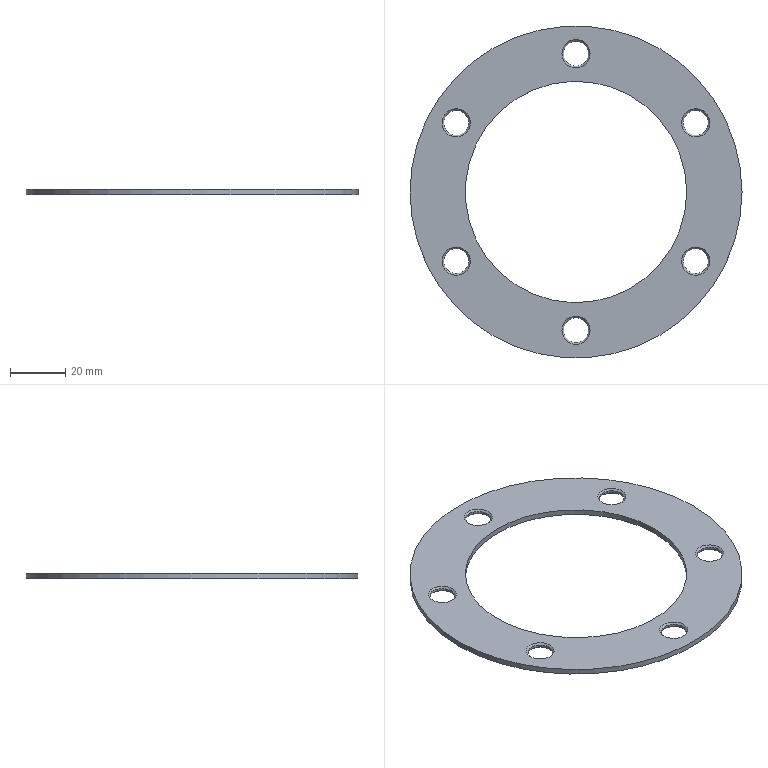Part | NX | 1 solid | 22 faces | box 120 x 120 x 2 mm | volume 11739 mm3 | cone 12 | cylinder 8 | plane 2 | commonest cylinder face diameters 9 x6 80 x1 120 x1
STEP:
#1=CARTESIAN_POINT('',(-41.051,28.897,1.4));
#2=VERTEX_POINT('',#1);
#3=CARTESIAN_POINT('',(-43.301,25.,1.4));
#4=DIRECTION('',(0.,0.,1.));
#5=DIRECTION('',(0.5,0.866,0.));
#6=AXIS2_PLACEMENT_3D('',#3,#4,#5);
#7=CIRCLE('',#6,4.5);
#8=EDGE_CURVE('',#2,#2,#7,.T.);
#9=ORIENTED_EDGE('',*,*,#8,.T.);
#10=EDGE_LOOP('',(#9));
#11=FACE_BOUND('',#10,.T.);
#12=CARTESIAN_POINT('',(-41.051,28.897,0.6));
#13=VERTEX_POINT('',#12);
#14=CARTESIAN_POINT('',(-43.301,25.,0.6));
#15=DIRECTION('',(0.,0.,-1.));
#16=DIRECTION('',(0.5,0.866,0.));
#17=AXIS2_PLACEMENT_3D('',#14,#15,#16);
#18=CIRCLE('',#17,4.5);
#19=EDGE_CURVE('',#13,#13,#18,.T.);
#20=ORIENTED_EDGE('',*,*,#19,.T.);
#21=EDGE_LOOP('',(#20));
#22=FACE_BOUND('',#21,.T.);
#23=CARTESIAN_POINT('',(-43.301,25.,0.));
#24=DIRECTION('',(0.,0.,1.));
#25=DIRECTION('',(-0.5,-0.866,0.));
#26=AXIS2_PLACEMENT_3D('',#23,#24,#25);
#27=CYLINDRICAL_SURFACE('',#26,4.5);
#28=ADVANCED_FACE('',(#11,#22),#27,.F.);
#29=CARTESIAN_POINT('',(-40.751,29.417,2.));
#30=VERTEX_POINT('',#29);
#31=CARTESIAN_POINT('',(-43.301,25.,2.));
#32=DIRECTION('',(0.,0.,-1.));
#33=DIRECTION('',(0.5,0.866,0.));
#34=AXIS2_PLACEMENT_3D('',#31,#32,#33);
#35=CIRCLE('',#34,5.1);
#36=EDGE_CURVE('',#30,#30,#35,.T.);
#37=ORIENTED_EDGE('',*,*,#36,.F.);
#38=EDGE_LOOP('',(#37));
#39=FACE_BOUND('',#38,.T.);
#40=ORIENTED_EDGE('',*,*,#8,.F.);
#41=EDGE_LOOP('',(#40));
#42=FACE_BOUND('',#41,.T.);
#43=CARTESIAN_POINT('',(-43.301,25.,1.4));
#44=DIRECTION('',(0.,0.,1.));
#45=DIRECTION('',(-0.5,-0.866,0.));
#46=AXIS2_PLACEMENT_3D('',#43,#44,#45);
#47=CONICAL_SURFACE('',#46,4.5,45.);
#48=ADVANCED_FACE('',(#39,#42),#47,.F.);
#49=ORIENTED_EDGE('',*,*,#19,.F.);
#50=EDGE_LOOP('',(#49));
#51=FACE_BOUND('',#50,.T.);
#52=CARTESIAN_POINT('',(-40.751,29.417,0.));
#53=VERTEX_POINT('',#52);
#54=CARTESIAN_POINT('',(-43.301,25.,0.));
#55=DIRECTION('',(0.,0.,1.));
#56=DIRECTION('',(0.5,0.866,0.));
#57=AXIS2_PLACEMENT_3D('',#54,#55,#56);
#58=CIRCLE('',#57,5.1);
#59=EDGE_CURVE('',#53,#53,#58,.T.);
#60=ORIENTED_EDGE('',*,*,#59,.F.);
#61=EDGE_LOOP('',(#60));
#62=FACE_BOUND('',#61,.T.);
#63=CARTESIAN_POINT('',(-43.301,25.,0.));
#64=DIRECTION('',(0.,0.,-1.));
#65=DIRECTION('',(0.5,0.866,0.));
#66=AXIS2_PLACEMENT_3D('',#63,#64,#65);
#67=CONICAL_SURFACE('',#66,5.1,45.);
#68=ADVANCED_FACE('',(#51,#62),#67,.F.);
#69=CARTESIAN_POINT('',(-45.551,-21.103,1.4));
#70=VERTEX_POINT('',#69);
#71=CARTESIAN_POINT('',(-43.301,-25.,1.4));
#72=DIRECTION('',(0.,0.,1.));
#73=DIRECTION('',(-0.5,0.866,0.));
#74=AXIS2_PLACEMENT_3D('',#71,#72,#73);
#75=CIRCLE('',#74,4.5);
#76=EDGE_CURVE('',#70,#70,#75,.T.);
#77=ORIENTED_EDGE('',*,*,#76,.T.);
#78=EDGE_LOOP('',(#77));
#79=FACE_BOUND('',#78,.T.);
#80=CARTESIAN_POINT('',(-45.551,-21.103,0.6));
#81=VERTEX_POINT('',#80);
#82=CARTESIAN_POINT('',(-43.301,-25.,0.6));
#83=DIRECTION('',(0.,0.,-1.));
#84=DIRECTION('',(-0.5,0.866,0.));
#85=AXIS2_PLACEMENT_3D('',#82,#83,#84);
#86=CIRCLE('',#85,4.5);
#87=EDGE_CURVE('',#81,#81,#86,.T.);
#88=ORIENTED_EDGE('',*,*,#87,.T.);
#89=EDGE_LOOP('',(#88));
#90=FACE_BOUND('',#89,.T.);
#91=CARTESIAN_POINT('',(-43.301,-25.,0.));
#92=DIRECTION('',(0.,0.,1.));
#93=DIRECTION('',(0.5,-0.866,0.));
#94=AXIS2_PLACEMENT_3D('',#91,#92,#93);
#95=CYLINDRICAL_SURFACE('',#94,4.5);
#96=ADVANCED_FACE('',(#79,#90),#95,.F.);
#97=CARTESIAN_POINT('',(-45.851,-20.583,2.));
#98=VERTEX_POINT('',#97);
#99=CARTESIAN_POINT('',(-43.301,-25.,2.));
#100=DIRECTION('',(0.,0.,-1.));
#101=DIRECTION('',(-0.5,0.866,0.));
#102=AXIS2_PLACEMENT_3D('',#99,#100,#101);
#103=CIRCLE('',#102,5.1);
#104=EDGE_CURVE('',#98,#98,#103,.T.);
#105=ORIENTED_EDGE('',*,*,#104,.F.);
#106=EDGE_LOOP('',(#105));
#107=FACE_BOUND('',#106,.T.);
#108=ORIENTED_EDGE('',*,*,#76,.F.);
#109=EDGE_LOOP('',(#108));
#110=FACE_BOUND('',#109,.T.);
#111=CARTESIAN_POINT('',(-43.301,-25.,1.4));
#112=DIRECTION('',(0.,0.,1.));
#113=DIRECTION('',(0.5,-0.866,0.));
#114=AXIS2_PLACEMENT_3D('',#111,#112,#113);
#115=CONICAL_SURFACE('',#114,4.5,45.);
#116=ADVANCED_FACE('',(#107,#110),#115,.F.);
#117=ORIENTED_EDGE('',*,*,#87,.F.);
#118=EDGE_LOOP('',(#117));
#119=FACE_BOUND('',#118,.T.);
#120=CARTESIAN_POINT('',(-45.851,-20.583,0.));
#121=VERTEX_POINT('',#120);
#122=CARTESIAN_POINT('',(-43.301,-25.,0.));
#123=DIRECTION('',(0.,0.,1.));
#124=DIRECTION('',(-0.5,0.866,0.));
#125=AXIS2_PLACEMENT_3D('',#122,#123,#124);
#126=CIRCLE('',#125,5.1);
#127=EDGE_CURVE('',#121,#121,#126,.T.);
#128=ORIENTED_EDGE('',*,*,#127,.F.);
#129=EDGE_LOOP('',(#128));
#130=FACE_BOUND('',#129,.T.);
#131=CARTESIAN_POINT('',(-43.301,-25.,0.));
#132=DIRECTION('',(0.,0.,-1.));
#133=DIRECTION('',(-0.5,0.866,0.));
#134=AXIS2_PLACEMENT_3D('',#131,#132,#133);
#135=CONICAL_SURFACE('',#134,5.1,45.);
#136=ADVANCED_FACE('',(#119,#130),#135,.F.);
#137=CARTESIAN_POINT('',(-4.5,-50.,1.4));
#138=VERTEX_POINT('',#137);
#139=CARTESIAN_POINT('',(0.,-50.,1.4));
#140=DIRECTION('',(0.,0.,1.));
#141=DIRECTION('',(-1.,0.,0.));
#142=AXIS2_PLACEMENT_3D('',#139,#140,#141);
#143=CIRCLE('',#142,4.5);
#144=EDGE_CURVE('',#138,#138,#143,.T.);
#145=ORIENTED_EDGE('',*,*,#144,.T.);
#146=EDGE_LOOP('',(#145));
#147=FACE_BOUND('',#146,.T.);
#148=CARTESIAN_POINT('',(-4.5,-50.,0.6));
#149=VERTEX_POINT('',#148);
#150=CARTESIAN_POINT('',(0.,-50.,0.6));
#151=DIRECTION('',(0.,0.,-1.));
#152=DIRECTION('',(-1.,0.,0.));
#153=AXIS2_PLACEMENT_3D('',#150,#151,#152);
#154=CIRCLE('',#153,4.5);
#155=EDGE_CURVE('',#149,#149,#154,.T.);
#156=ORIENTED_EDGE('',*,*,#155,.T.);
#157=EDGE_LOOP('',(#156));
#158=FACE_BOUND('',#157,.T.);
#159=CARTESIAN_POINT('',(0.,-50.,0.));
#160=DIRECTION('',(0.,0.,1.));
#161=DIRECTION('',(1.,0.,0.));
#162=AXIS2_PLACEMENT_3D('',#159,#160,#161);
#163=CYLINDRICAL_SURFACE('',#162,4.5);
#164=ADVANCED_FACE('',(#147,#158),#163,.F.);
#165=CARTESIAN_POINT('',(-5.1,-50.,2.));
#166=VERTEX_POINT('',#165);
#167=CARTESIAN_POINT('',(0.,-50.,2.));
#168=DIRECTION('',(0.,0.,-1.));
#169=DIRECTION('',(-1.,0.,0.));
#170=AXIS2_PLACEMENT_3D('',#167,#168,#169);
#171=CIRCLE('',#170,5.1);
#172=EDGE_CURVE('',#166,#166,#171,.T.);
#173=ORIENTED_EDGE('',*,*,#172,.F.);
#174=EDGE_LOOP('',(#173));
#175=FACE_BOUND('',#174,.T.);
#176=ORIENTED_EDGE('',*,*,#144,.F.);
#177=EDGE_LOOP('',(#176));
#178=FACE_BOUND('',#177,.T.);
#179=CARTESIAN_POINT('',(0.,-50.,1.4));
#180=DIRECTION('',(0.,0.,1.));
#181=DIRECTION('',(1.,0.,0.));
#182=AXIS2_PLACEMENT_3D('',#179,#180,#181);
#183=CONICAL_SURFACE('',#182,4.5,45.);
#184=ADVANCED_FACE('',(#175,#178),#183,.F.);
#185=ORIENTED_EDGE('',*,*,#155,.F.);
#186=EDGE_LOOP('',(#185));
#187=FACE_BOUND('',#186,.T.);
#188=CARTESIAN_POINT('',(-5.1,-50.,0.));
#189=VERTEX_POINT('',#188);
#190=CARTESIAN_POINT('',(0.,-50.,0.));
#191=DIRECTION('',(0.,0.,1.));
#192=DIRECTION('',(-1.,0.,0.));
#193=AXIS2_PLACEMENT_3D('',#190,#191,#192);
#194=CIRCLE('',#193,5.1);
#195=EDGE_CURVE('',#189,#189,#194,.T.);
#196=ORIENTED_EDGE('',*,*,#195,.F.);
#197=EDGE_LOOP('',(#196));
#198=FACE_BOUND('',#197,.T.);
#199=CARTESIAN_POINT('',(0.,-50.,0.));
#200=DIRECTION('',(0.,0.,-1.));
#201=DIRECTION('',(-1.,0.,0.));
#202=AXIS2_PLACEMENT_3D('',#199,#200,#201);
#203=CONICAL_SURFACE('',#202,5.1,45.);
#204=ADVANCED_FACE('',(#187,#198),#203,.F.);
#205=CARTESIAN_POINT('',(41.051,-28.897,1.4));
#206=VERTEX_POINT('',#205);
#207=CARTESIAN_POINT('',(43.301,-25.,1.4));
#208=DIRECTION('',(0.,0.,1.));
#209=DIRECTION('',(-0.5,-0.866,0.));
#210=AXIS2_PLACEMENT_3D('',#207,#208,#209);
#211=CIRCLE('',#210,4.5);
#212=EDGE_CURVE('',#206,#206,#211,.T.);
#213=ORIENTED_EDGE('',*,*,#212,.T.);
#214=EDGE_LOOP('',(#213));
#215=FACE_BOUND('',#214,.T.);
#216=CARTESIAN_POINT('',(41.051,-28.897,0.6));
#217=VERTEX_POINT('',#216);
#218=CARTESIAN_POINT('',(43.301,-25.,0.6));
#219=DIRECTION('',(0.,0.,-1.));
#220=DIRECTION('',(-0.5,-0.866,0.));
#221=AXIS2_PLACEMENT_3D('',#218,#219,#220);
#222=CIRCLE('',#221,4.5);
#223=EDGE_CURVE('',#217,#217,#222,.T.);
#224=ORIENTED_EDGE('',*,*,#223,.T.);
#225=EDGE_LOOP('',(#224));
#226=FACE_BOUND('',#225,.T.);
#227=CARTESIAN_POINT('',(43.301,-25.,0.));
#228=DIRECTION('',(0.,0.,1.));
#229=DIRECTION('',(0.5,0.866,0.));
#230=AXIS2_PLACEMENT_3D('',#227,#228,#229);
#231=CYLINDRICAL_SURFACE('',#230,4.5);
#232=ADVANCED_FACE('',(#215,#226),#231,.F.);
#233=CARTESIAN_POINT('',(40.751,-29.417,2.));
#234=VERTEX_POINT('',#233);
#235=CARTESIAN_POINT('',(43.301,-25.,2.));
#236=DIRECTION('',(0.,0.,-1.));
#237=DIRECTION('',(-0.5,-0.866,0.));
#238=AXIS2_PLACEMENT_3D('',#235,#236,#237);
#239=CIRCLE('',#238,5.1);
#240=EDGE_CURVE('',#234,#234,#239,.T.);
#241=ORIENTED_EDGE('',*,*,#240,.F.);
#242=EDGE_LOOP('',(#241));
#243=FACE_BOUND('',#242,.T.);
#244=ORIENTED_EDGE('',*,*,#212,.F.);
#245=EDGE_LOOP('',(#244));
#246=FACE_BOUND('',#245,.T.);
#247=CARTESIAN_POINT('',(43.301,-25.,1.4));
#248=DIRECTION('',(0.,0.,1.));
#249=DIRECTION('',(0.5,0.866,0.));
#250=AXIS2_PLACEMENT_3D('',#247,#248,#249);
#251=CONICAL_SURFACE('',#250,4.5,45.);
#252=ADVANCED_FACE('',(#243,#246),#251,.F.);
#253=ORIENTED_EDGE('',*,*,#223,.F.);
#254=EDGE_LOOP('',(#253));
#255=FACE_BOUND('',#254,.T.);
#256=CARTESIAN_POINT('',(40.751,-29.417,0.));
#257=VERTEX_POINT('',#256);
#258=CARTESIAN_POINT('',(43.301,-25.,0.));
#259=DIRECTION('',(0.,0.,1.));
#260=DIRECTION('',(-0.5,-0.866,0.));
#261=AXIS2_PLACEMENT_3D('',#258,#259,#260);
#262=CIRCLE('',#261,5.1);
#263=EDGE_CURVE('',#257,#257,#262,.T.);
#264=ORIENTED_EDGE('',*,*,#263,.F.);
#265=EDGE_LOOP('',(#264));
#266=FACE_BOUND('',#265,.T.);
#267=CARTESIAN_POINT('',(43.301,-25.,0.));
#268=DIRECTION('',(0.,0.,-1.));
#269=DIRECTION('',(-0.5,-0.866,0.));
#270=AXIS2_PLACEMENT_3D('',#267,#268,#269);
#271=CONICAL_SURFACE('',#270,5.1,45.);
#272=ADVANCED_FACE('',(#255,#266),#271,.F.);
#273=CARTESIAN_POINT('',(45.551,21.103,1.4));
#274=VERTEX_POINT('',#273);
#275=CARTESIAN_POINT('',(43.301,25.,1.4));
#276=DIRECTION('',(0.,0.,1.));
#277=DIRECTION('',(0.5,-0.866,0.));
#278=AXIS2_PLACEMENT_3D('',#275,#276,#277);
#279=CIRCLE('',#278,4.5);
#280=EDGE_CURVE('',#274,#274,#279,.T.);
#281=ORIENTED_EDGE('',*,*,#280,.T.);
#282=EDGE_LOOP('',(#281));
#283=FACE_BOUND('',#282,.T.);
#284=CARTESIAN_POINT('',(45.551,21.103,0.6));
#285=VERTEX_POINT('',#284);
#286=CARTESIAN_POINT('',(43.301,25.,0.6));
#287=DIRECTION('',(0.,0.,-1.));
#288=DIRECTION('',(0.5,-0.866,0.));
#289=AXIS2_PLACEMENT_3D('',#286,#287,#288);
#290=CIRCLE('',#289,4.5);
#291=EDGE_CURVE('',#285,#285,#290,.T.);
#292=ORIENTED_EDGE('',*,*,#291,.T.);
#293=EDGE_LOOP('',(#292));
#294=FACE_BOUND('',#293,.T.);
#295=CARTESIAN_POINT('',(43.301,25.,0.));
#296=DIRECTION('',(0.,0.,1.));
#297=DIRECTION('',(-0.5,0.866,0.));
#298=AXIS2_PLACEMENT_3D('',#295,#296,#297);
#299=CYLINDRICAL_SURFACE('',#298,4.5);
#300=ADVANCED_FACE('',(#283,#294),#299,.F.);
#301=CARTESIAN_POINT('',(45.851,20.583,2.));
#302=VERTEX_POINT('',#301);
#303=CARTESIAN_POINT('',(43.301,25.,2.));
#304=DIRECTION('',(0.,0.,-1.));
#305=DIRECTION('',(0.5,-0.866,0.));
#306=AXIS2_PLACEMENT_3D('',#303,#304,#305);
#307=CIRCLE('',#306,5.1);
#308=EDGE_CURVE('',#302,#302,#307,.T.);
#309=ORIENTED_EDGE('',*,*,#308,.F.);
#310=EDGE_LOOP('',(#309));
#311=FACE_BOUND('',#310,.T.);
#312=ORIENTED_EDGE('',*,*,#280,.F.);
#313=EDGE_LOOP('',(#312));
#314=FACE_BOUND('',#313,.T.);
#315=CARTESIAN_POINT('',(43.301,25.,1.4));
#316=DIRECTION('',(0.,0.,1.));
#317=DIRECTION('',(-0.5,0.866,0.));
#318=AXIS2_PLACEMENT_3D('',#315,#316,#317);
#319=CONICAL_SURFACE('',#318,4.5,45.);
#320=ADVANCED_FACE('',(#311,#314),#319,.F.);
#321=ORIENTED_EDGE('',*,*,#291,.F.);
#322=EDGE_LOOP('',(#321));
#323=FACE_BOUND('',#322,.T.);
#324=CARTESIAN_POINT('',(45.851,20.583,0.));
#325=VERTEX_POINT('',#324);
#326=CARTESIAN_POINT('',(43.301,25.,0.));
#327=DIRECTION('',(0.,0.,1.));
#328=DIRECTION('',(0.5,-0.866,0.));
#329=AXIS2_PLACEMENT_3D('',#326,#327,#328);
#330=CIRCLE('',#329,5.1);
#331=EDGE_CURVE('',#325,#325,#330,.T.);
#332=ORIENTED_EDGE('',*,*,#331,.F.);
#333=EDGE_LOOP('',(#332));
#334=FACE_BOUND('',#333,.T.);
#335=CARTESIAN_POINT('',(43.301,25.,0.));
#336=DIRECTION('',(0.,0.,-1.));
#337=DIRECTION('',(0.5,-0.866,0.));
#338=AXIS2_PLACEMENT_3D('',#335,#336,#337);
#339=CONICAL_SURFACE('',#338,5.1,45.);
#340=ADVANCED_FACE('',(#323,#334),#339,.F.);
#341=CARTESIAN_POINT('',(60.,0.,2.));
#342=VERTEX_POINT('',#341);
#343=CARTESIAN_POINT('',(0.,0.,2.));
#344=DIRECTION('',(0.,0.,1.));
#345=DIRECTION('',(1.,0.,0.));
#346=AXIS2_PLACEMENT_3D('',#343,#344,#345);
#347=CIRCLE('',#346,60.);
#348=EDGE_CURVE('',#342,#342,#347,.T.);
#349=ORIENTED_EDGE('',*,*,#348,.F.);
#350=EDGE_LOOP('',(#349));
#351=FACE_BOUND('',#350,.T.);
#352=CARTESIAN_POINT('',(60.,0.,0.));
#353=VERTEX_POINT('',#352);
#354=CARTESIAN_POINT('',(0.,0.,0.));
#355=DIRECTION('',(0.,0.,1.));
#356=DIRECTION('',(1.,0.,0.));
#357=AXIS2_PLACEMENT_3D('',#354,#355,#356);
#358=CIRCLE('',#357,60.);
#359=EDGE_CURVE('',#353,#353,#358,.T.);
#360=ORIENTED_EDGE('',*,*,#359,.T.);
#361=EDGE_LOOP('',(#360));
#362=FACE_BOUND('',#361,.T.);
#363=CARTESIAN_POINT('',(0.,0.,2.));
#364=DIRECTION('',(0.,0.,-1.));
#365=DIRECTION('',(1.,0.,0.));
#366=AXIS2_PLACEMENT_3D('',#363,#364,#365);
#367=CYLINDRICAL_SURFACE('',#366,60.);
#368=ADVANCED_FACE('',(#351,#362),#367,.T.);
#369=CARTESIAN_POINT('',(40.,0.,2.));
#370=VERTEX_POINT('',#369);
#371=CARTESIAN_POINT('',(0.,0.,2.));
#372=DIRECTION('',(0.,0.,1.));
#373=DIRECTION('',(1.,0.,0.));
#374=AXIS2_PLACEMENT_3D('',#371,#372,#373);
#375=CIRCLE('',#374,40.);
#376=EDGE_CURVE('',#370,#370,#375,.T.);
#377=ORIENTED_EDGE('',*,*,#376,.T.);
#378=EDGE_LOOP('',(#377));
#379=FACE_BOUND('',#378,.T.);
#380=CARTESIAN_POINT('',(40.,0.,0.));
#381=VERTEX_POINT('',#380);
#382=CARTESIAN_POINT('',(0.,0.,0.));
#383=DIRECTION('',(0.,0.,1.));
#384=DIRECTION('',(1.,0.,0.));
#385=AXIS2_PLACEMENT_3D('',#382,#383,#384);
#386=CIRCLE('',#385,40.);
#387=EDGE_CURVE('',#381,#381,#386,.T.);
#388=ORIENTED_EDGE('',*,*,#387,.F.);
#389=EDGE_LOOP('',(#388));
#390=FACE_BOUND('',#389,.T.);
#391=CARTESIAN_POINT('',(0.,0.,2.));
#392=DIRECTION('',(0.,0.,-1.));
#393=DIRECTION('',(1.,0.,0.));
#394=AXIS2_PLACEMENT_3D('',#391,#392,#393);
#395=CYLINDRICAL_SURFACE('',#394,40.);
#396=ADVANCED_FACE('',(#379,#390),#395,.F.);
#397=ORIENTED_EDGE('',*,*,#36,.T.);
#398=EDGE_LOOP('',(#397));
#399=FACE_BOUND('',#398,.T.);
#400=ORIENTED_EDGE('',*,*,#104,.T.);
#401=EDGE_LOOP('',(#400));
#402=FACE_BOUND('',#401,.T.);
#403=ORIENTED_EDGE('',*,*,#172,.T.);
#404=EDGE_LOOP('',(#403));
#405=FACE_BOUND('',#404,.T.);
#406=ORIENTED_EDGE('',*,*,#240,.T.);
#407=EDGE_LOOP('',(#406));
#408=FACE_BOUND('',#407,.T.);
#409=ORIENTED_EDGE('',*,*,#308,.T.);
#410=EDGE_LOOP('',(#409));
#411=FACE_BOUND('',#410,.T.);
#412=CARTESIAN_POINT('',(5.1,50.,2.));
#413=VERTEX_POINT('',#412);
#414=CARTESIAN_POINT('',(0.,50.,2.));
#415=DIRECTION('',(0.,0.,-1.));
#416=DIRECTION('',(1.,0.,0.));
#417=AXIS2_PLACEMENT_3D('',#414,#415,#416);
#418=CIRCLE('',#417,5.1);
#419=EDGE_CURVE('',#413,#413,#418,.T.);
#420=ORIENTED_EDGE('',*,*,#419,.T.);
#421=EDGE_LOOP('',(#420));
#422=FACE_BOUND('',#421,.T.);
#423=ORIENTED_EDGE('',*,*,#348,.T.);
#424=EDGE_LOOP('',(#423));
#425=FACE_BOUND('',#424,.T.);
#426=ORIENTED_EDGE('',*,*,#376,.F.);
#427=EDGE_LOOP('',(#426));
#428=FACE_BOUND('',#427,.T.);
#429=CARTESIAN_POINT('',(0.,0.,2.));
#430=DIRECTION('',(0.,0.,1.));
#431=DIRECTION('',(-1.,0.,0.));
#432=AXIS2_PLACEMENT_3D('',#429,#430,#431);
#433=PLANE('',#432);
#434=ADVANCED_FACE('',(#399,#402,#405,#408,#411,#422,#425,#428),#433,.T.);
#435=ORIENTED_EDGE('',*,*,#59,.T.);
#436=EDGE_LOOP('',(#435));
#437=FACE_BOUND('',#436,.T.);
#438=ORIENTED_EDGE('',*,*,#127,.T.);
#439=EDGE_LOOP('',(#438));
#440=FACE_BOUND('',#439,.T.);
#441=ORIENTED_EDGE('',*,*,#195,.T.);
#442=EDGE_LOOP('',(#441));
#443=FACE_BOUND('',#442,.T.);
#444=ORIENTED_EDGE('',*,*,#263,.T.);
#445=EDGE_LOOP('',(#444));
#446=FACE_BOUND('',#445,.T.);
#447=ORIENTED_EDGE('',*,*,#331,.T.);
#448=EDGE_LOOP('',(#447));
#449=FACE_BOUND('',#448,.T.);
#450=CARTESIAN_POINT('',(5.1,50.,0.));
#451=VERTEX_POINT('',#450);
#452=CARTESIAN_POINT('',(0.,50.,0.));
#453=DIRECTION('',(0.,0.,1.));
#454=DIRECTION('',(1.,0.,0.));
#455=AXIS2_PLACEMENT_3D('',#452,#453,#454);
#456=CIRCLE('',#455,5.1);
#457=EDGE_CURVE('',#451,#451,#456,.T.);
#458=ORIENTED_EDGE('',*,*,#457,.T.);
#459=EDGE_LOOP('',(#458));
#460=FACE_BOUND('',#459,.T.);
#461=ORIENTED_EDGE('',*,*,#359,.F.);
#462=EDGE_LOOP('',(#461));
#463=FACE_BOUND('',#462,.T.);
#464=ORIENTED_EDGE('',*,*,#387,.T.);
#465=EDGE_LOOP('',(#464));
#466=FACE_BOUND('',#465,.T.);
#467=CARTESIAN_POINT('',(0.,0.,0.));
#468=DIRECTION('',(0.,0.,1.));
#469=DIRECTION('',(-1.,0.,0.));
#470=AXIS2_PLACEMENT_3D('',#467,#468,#469);
#471=PLANE('',#470);
#472=ADVANCED_FACE('',(#437,#440,#443,#446,#449,#460,#463,#466),#471,.F.);
#473=CARTESIAN_POINT('',(4.5,50.,1.4));
#474=VERTEX_POINT('',#473);
#475=CARTESIAN_POINT('',(0.,50.,1.4));
#476=DIRECTION('',(0.,0.,1.));
#477=DIRECTION('',(1.,0.,0.));
#478=AXIS2_PLACEMENT_3D('',#475,#476,#477);
#479=CIRCLE('',#478,4.5);
#480=EDGE_CURVE('',#474,#474,#479,.T.);
#481=ORIENTED_EDGE('',*,*,#480,.T.);
#482=EDGE_LOOP('',(#481));
#483=FACE_BOUND('',#482,.T.);
#484=CARTESIAN_POINT('',(4.5,50.,0.6));
#485=VERTEX_POINT('',#484);
#486=CARTESIAN_POINT('',(0.,50.,0.6));
#487=DIRECTION('',(0.,0.,-1.));
#488=DIRECTION('',(1.,0.,0.));
#489=AXIS2_PLACEMENT_3D('',#486,#487,#488);
#490=CIRCLE('',#489,4.5);
#491=EDGE_CURVE('',#485,#485,#490,.T.);
#492=ORIENTED_EDGE('',*,*,#491,.T.);
#493=EDGE_LOOP('',(#492));
#494=FACE_BOUND('',#493,.T.);
#495=CARTESIAN_POINT('',(0.,50.,0.));
#496=DIRECTION('',(0.,0.,1.));
#497=DIRECTION('',(-1.,0.,0.));
#498=AXIS2_PLACEMENT_3D('',#495,#496,#497);
#499=CYLINDRICAL_SURFACE('',#498,4.5);
#500=ADVANCED_FACE('',(#483,#494),#499,.F.);
#501=ORIENTED_EDGE('',*,*,#491,.F.);
#502=EDGE_LOOP('',(#501));
#503=FACE_BOUND('',#502,.T.);
#504=ORIENTED_EDGE('',*,*,#457,.F.);
#505=EDGE_LOOP('',(#504));
#506=FACE_BOUND('',#505,.T.);
#507=CARTESIAN_POINT('',(0.,50.,0.));
#508=DIRECTION('',(0.,0.,-1.));
#509=DIRECTION('',(1.,0.,0.));
#510=AXIS2_PLACEMENT_3D('',#507,#508,#509);
#511=CONICAL_SURFACE('',#510,5.1,45.);
#512=ADVANCED_FACE('',(#503,#506),#511,.F.);
#513=ORIENTED_EDGE('',*,*,#419,.F.);
#514=EDGE_LOOP('',(#513));
#515=FACE_BOUND('',#514,.T.);
#516=ORIENTED_EDGE('',*,*,#480,.F.);
#517=EDGE_LOOP('',(#516));
#518=FACE_BOUND('',#517,.T.);
#519=CARTESIAN_POINT('',(0.,50.,1.4));
#520=DIRECTION('',(0.,0.,1.));
#521=DIRECTION('',(-1.,0.,0.));
#522=AXIS2_PLACEMENT_3D('',#519,#520,#521);
#523=CONICAL_SURFACE('',#522,4.5,45.);
#524=ADVANCED_FACE('',(#515,#518),#523,.F.);
#525=CLOSED_SHELL('',(#28,#48,#68,#96,#116,#136,#164,#184,#204,#232,#252,#272,#300,#320,#340,#368,#396,#434,#472,#500,#512,#524));
#526=MANIFOLD_SOLID_BREP('',#525);
#527=(LENGTH_UNIT()NAMED_UNIT(*)SI_UNIT(.MILLI.,.METRE.));
#528=UNCERTAINTY_MEASURE_WITH_UNIT(LENGTH_MEASURE(0.00002),#527,'','');
#529=(NAMED_UNIT(*)PLANE_ANGLE_UNIT()SI_UNIT($,.RADIAN.));
#530=PLANE_ANGLE_MEASURE_WITH_UNIT(PLANE_ANGLE_MEASURE(0.01745),#529);
#531=DIMENSIONAL_EXPONENTS(0.,0.,0.,0.,0.,0.,0.);
#532=(CONVERSION_BASED_UNIT('DEGREE',#530)NAMED_UNIT(#531)PLANE_ANGLE_UNIT());
#533=(NAMED_UNIT(*)SI_UNIT($,.STERADIAN.)SOLID_ANGLE_UNIT());
#534=(GEOMETRIC_REPRESENTATION_CONTEXT(3)GLOBAL_UNCERTAINTY_ASSIGNED_CONTEXT((#528))GLOBAL_UNIT_ASSIGNED_CONTEXT((#527,#532,#533))REPRESENTATION_CONTEXT('',''));
#535=ADVANCED_BREP_SHAPE_REPRESENTATION('',(#526),#534);